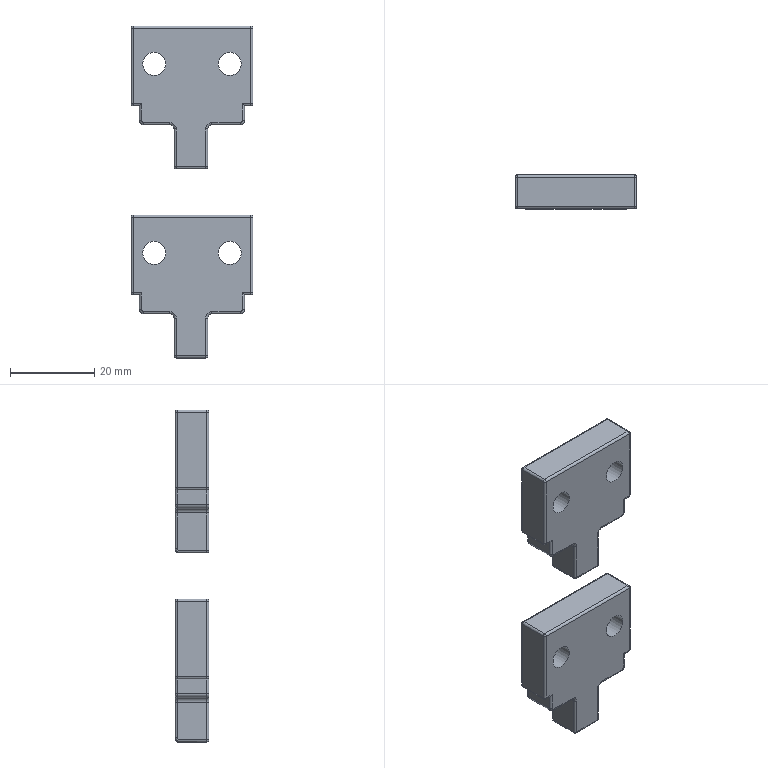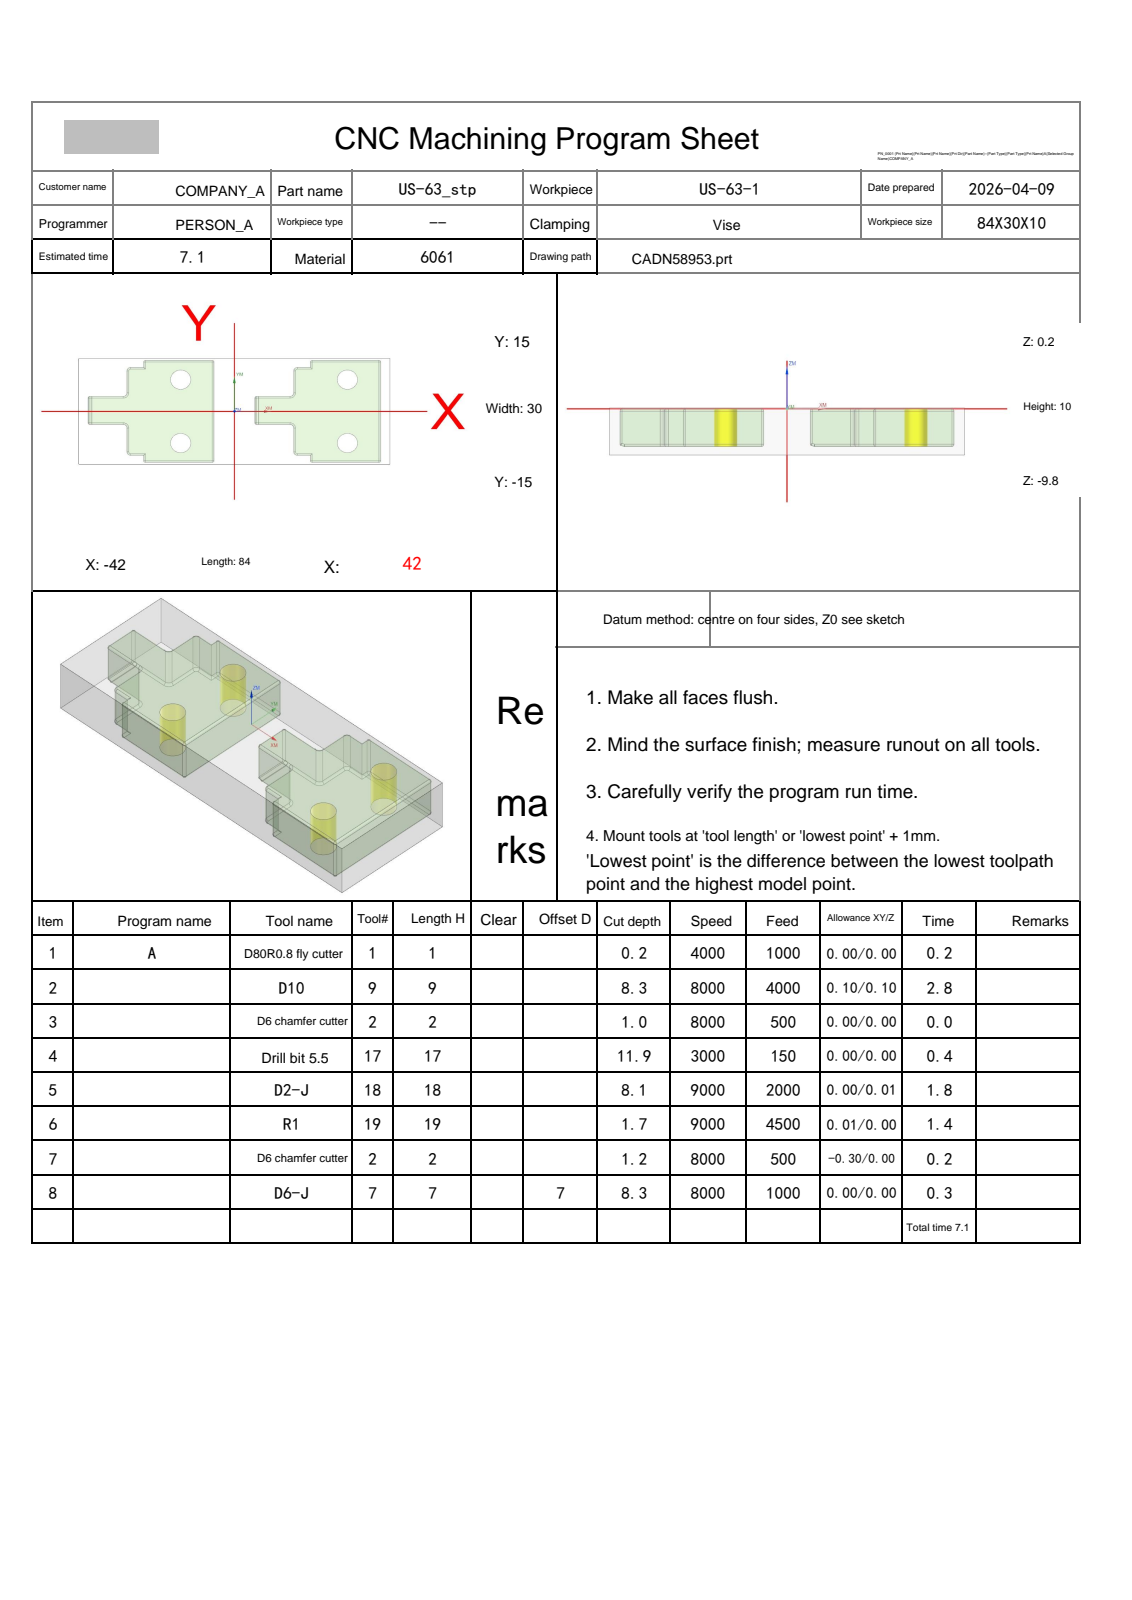NC program | NX | posted by the shop | part box 29 x 8 x 79 mm
Lines 2423 to 2454 of 24039:
N3 T02 M06
(D6 chamfer cutter  D=6. R=0. H=02 ce=0.00 di=0.10)
G00 G90 G54 X30.5 Y9. M03 S8000
G43 H02 Z20.
M08
G98 G81 X30.5 Y9. Z-.8 R1. F500.
Y-9.
X-14.5
Y9.
G80
G00 Z20.
G91 G28 Z0.0
M05
M09
G91 G28 Z0.0
M01
N4 T17 M06
(Drill bit 5.5 D=5.5 DR_a=118 H=17)
G00 G90 G54 X30.5 Y9. M03 S3000
G43 H17 Z20.
M08
G98 G83 X30.5 Y9. Z-11.652 R1. F150. Q3.
Y-9.
X-14.5
Y9.
G80
G00 Z20.
G91 G28 Z0.0
M05
M09
G91 G28 Z0.0
M01